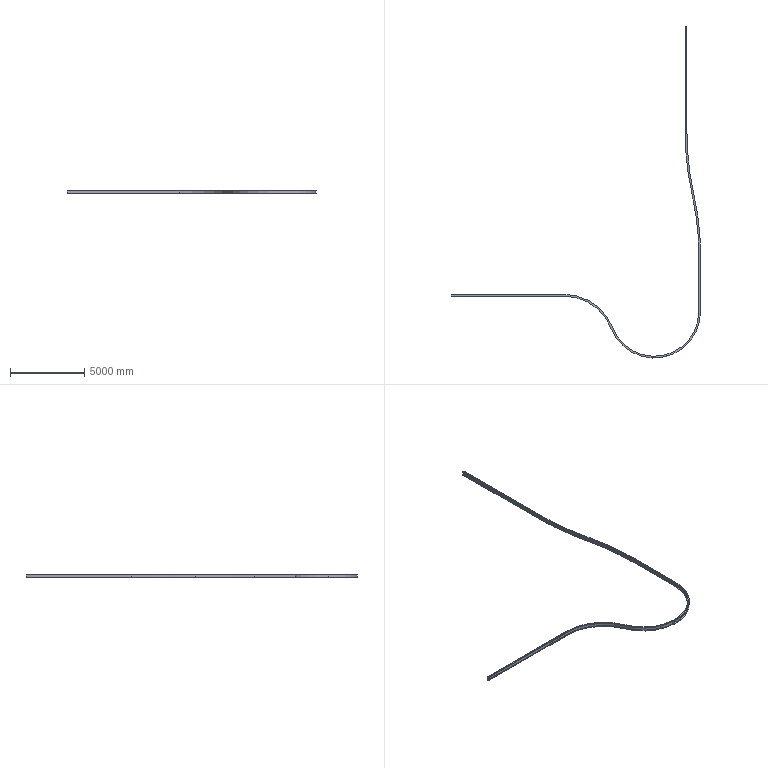Part | SolidWorks | features BaseBody 1 | 1 solid | 142 faces | box 16778 x 22359 x 250 mm | volume 204415095 mm3 | cylinder 48 | plane 46 | torus 32 | cone 16 | commonest cylinder face diameters 10 x12 20 x12 6006 x2 6242 x2 6797 x2 7033 x2